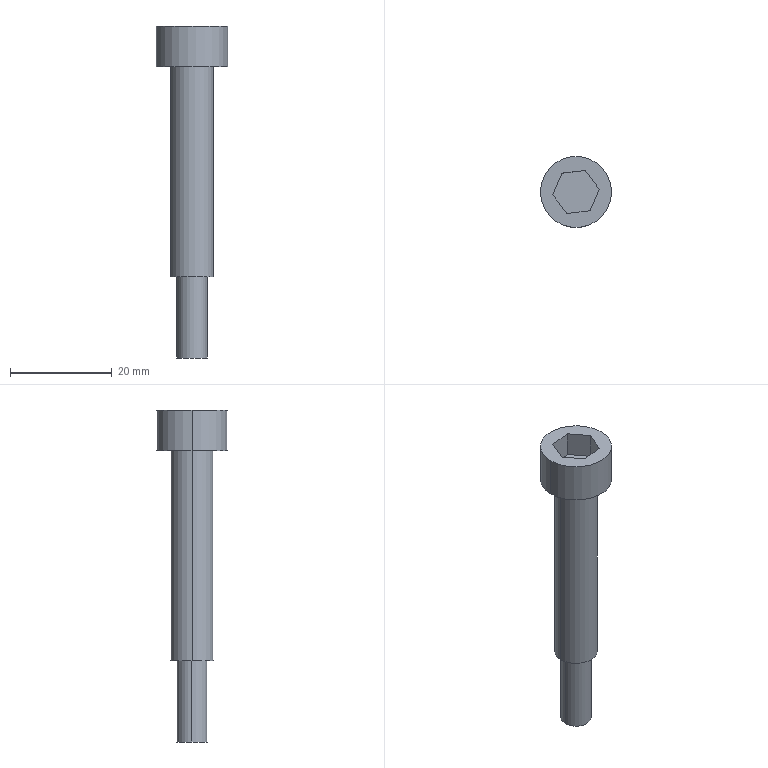Part | SolidWorks | features ICE 2, Cut 1, Extrusion 1 | 1 solid | 17 faces | box 14 x 14 x 65.4 mm | volume 3691 mm3 | plane 11 | cylinder 6 | commonest cylinder face diameters 6 x2 8.382 x2 14 x2
STEP:
#1=CARTESIAN_POINT('',(-29.159,-76.997,-57.4));
#2=VERTEX_POINT('',#1);
#3=CARTESIAN_POINT('',(-23.159,-76.997,-57.4));
#4=VERTEX_POINT('',#3);
#5=CARTESIAN_POINT('',(-26.159,-76.997,-57.4));
#6=DIRECTION('',(0.,0.,-1.));
#7=DIRECTION('',(0.,1.,0.));
#8=AXIS2_PLACEMENT_3D('',#5,#6,#7);
#9=CIRCLE('',#8,3.);
#10=EDGE_CURVE('',#2,#4,#9,.T.);
#11=ORIENTED_EDGE('',*,*,#10,.F.);
#12=CARTESIAN_POINT('',(-29.159,-76.997,-41.4));
#13=VERTEX_POINT('',#12);
#14=CARTESIAN_POINT('',(-29.159,-76.997,-65.885));
#15=DIRECTION('',(0.,0.,1.));
#16=VECTOR('',#15,1000.);
#17=LINE('',#14,#16);
#18=EDGE_CURVE('',#2,#13,#17,.T.);
#19=ORIENTED_EDGE('',*,*,#18,.T.);
#20=CARTESIAN_POINT('',(-23.159,-76.997,-41.4));
#21=VERTEX_POINT('',#20);
#22=CARTESIAN_POINT('',(-26.159,-76.997,-41.4));
#23=DIRECTION('',(0.,0.,-1.));
#24=DIRECTION('',(1.,0.,0.));
#25=AXIS2_PLACEMENT_3D('',#22,#23,#24);
#26=CIRCLE('',#25,3.);
#27=EDGE_CURVE('',#13,#21,#26,.T.);
#28=ORIENTED_EDGE('',*,*,#27,.T.);
#29=CARTESIAN_POINT('',(-23.159,-76.997,-65.885));
#30=DIRECTION('',(0.,0.,1.));
#31=VECTOR('',#30,1000.);
#32=LINE('',#29,#31);
#33=EDGE_CURVE('',#4,#21,#32,.T.);
#34=ORIENTED_EDGE('',*,*,#33,.F.);
#35=EDGE_LOOP('',(#11,#19,#28,#34));
#36=FACE_OUTER_BOUND('',#35,.T.);
#37=CARTESIAN_POINT('',(-26.159,-76.997,-65.885));
#38=DIRECTION('',(0.,0.,1.));
#39=DIRECTION('',(1.,0.,0.));
#40=AXIS2_PLACEMENT_3D('',#37,#38,#39);
#41=CYLINDRICAL_SURFACE('',#40,3.);
#42=ADVANCED_FACE('',(#36),#41,.T.);
#43=CARTESIAN_POINT('',(-21.968,-76.997,-41.4));
#44=VERTEX_POINT('',#43);
#45=CARTESIAN_POINT('',(-30.35,-76.997,-41.4));
#46=VERTEX_POINT('',#45);
#47=CARTESIAN_POINT('',(-26.159,-76.997,-41.4));
#48=DIRECTION('',(0.,0.,1.));
#49=DIRECTION('',(1.,0.,0.));
#50=AXIS2_PLACEMENT_3D('',#47,#48,#49);
#51=CIRCLE('',#50,4.191);
#52=EDGE_CURVE('',#44,#46,#51,.T.);
#53=ORIENTED_EDGE('',*,*,#52,.T.);
#54=CARTESIAN_POINT('',(-30.35,-76.997,0.));
#55=VERTEX_POINT('',#54);
#56=CARTESIAN_POINT('',(-30.35,-76.997,-53.254));
#57=DIRECTION('',(0.,0.,1.));
#58=VECTOR('',#57,1000.);
#59=LINE('',#56,#58);
#60=EDGE_CURVE('',#46,#55,#59,.T.);
#61=ORIENTED_EDGE('',*,*,#60,.T.);
#62=CARTESIAN_POINT('',(-21.968,-76.997,0.));
#63=VERTEX_POINT('',#62);
#64=CARTESIAN_POINT('',(-26.159,-76.997,0.));
#65=DIRECTION('',(0.,0.,-1.));
#66=DIRECTION('',(1.,0.,0.));
#67=AXIS2_PLACEMENT_3D('',#64,#65,#66);
#68=CIRCLE('',#67,4.191);
#69=EDGE_CURVE('',#55,#63,#68,.T.);
#70=ORIENTED_EDGE('',*,*,#69,.T.);
#71=CARTESIAN_POINT('',(-21.968,-76.997,-53.254));
#72=DIRECTION('',(0.,0.,1.));
#73=VECTOR('',#72,1000.);
#74=LINE('',#71,#73);
#75=EDGE_CURVE('',#44,#63,#74,.T.);
#76=ORIENTED_EDGE('',*,*,#75,.F.);
#77=EDGE_LOOP('',(#53,#61,#70,#76));
#78=FACE_OUTER_BOUND('',#77,.T.);
#79=CARTESIAN_POINT('',(-26.159,-76.997,-53.254));
#80=DIRECTION('',(0.,0.,1.));
#81=DIRECTION('',(1.,0.,0.));
#82=AXIS2_PLACEMENT_3D('',#79,#80,#81);
#83=CYLINDRICAL_SURFACE('',#82,4.191);
#84=ADVANCED_FACE('',(#78),#83,.T.);
#85=CARTESIAN_POINT('',(-19.159,-76.997,8.));
#86=VERTEX_POINT('',#85);
#87=CARTESIAN_POINT('',(-33.159,-76.997,8.));
#88=VERTEX_POINT('',#87);
#89=CARTESIAN_POINT('',(-26.159,-76.997,8.));
#90=DIRECTION('',(0.,0.,1.));
#91=DIRECTION('',(1.,0.,0.));
#92=AXIS2_PLACEMENT_3D('',#89,#90,#91);
#93=CIRCLE('',#92,7.);
#94=EDGE_CURVE('',#86,#88,#93,.T.);
#95=ORIENTED_EDGE('',*,*,#94,.F.);
#96=CARTESIAN_POINT('',(-19.159,-76.997,0.));
#97=VERTEX_POINT('',#96);
#98=CARTESIAN_POINT('',(-19.159,-76.997,8.));
#99=DIRECTION('',(0.,0.,-1.));
#100=VECTOR('',#99,1000.);
#101=LINE('',#98,#100);
#102=EDGE_CURVE('',#86,#97,#101,.T.);
#103=ORIENTED_EDGE('',*,*,#102,.T.);
#104=CARTESIAN_POINT('',(-33.159,-76.997,0.));
#105=VERTEX_POINT('',#104);
#106=CARTESIAN_POINT('',(-26.159,-76.997,0.));
#107=DIRECTION('',(0.,0.,1.));
#108=DIRECTION('',(1.,0.,0.));
#109=AXIS2_PLACEMENT_3D('',#106,#107,#108);
#110=CIRCLE('',#109,7.);
#111=EDGE_CURVE('',#97,#105,#110,.T.);
#112=ORIENTED_EDGE('',*,*,#111,.T.);
#113=CARTESIAN_POINT('',(-33.159,-76.997,8.));
#114=DIRECTION('',(0.,0.,-1.));
#115=VECTOR('',#114,1000.);
#116=LINE('',#113,#115);
#117=EDGE_CURVE('',#88,#105,#116,.T.);
#118=ORIENTED_EDGE('',*,*,#117,.F.);
#119=EDGE_LOOP('',(#95,#103,#112,#118));
#120=FACE_OUTER_BOUND('',#119,.T.);
#121=CARTESIAN_POINT('',(-26.159,-76.997,8.));
#122=DIRECTION('',(0.,0.,-1.));
#123=DIRECTION('',(-1.,0.,0.));
#124=AXIS2_PLACEMENT_3D('',#121,#122,#123);
#125=CYLINDRICAL_SURFACE('',#124,7.);
#126=ADVANCED_FACE('',(#120),#125,.T.);
#127=ORIENTED_EDGE('',*,*,#102,.F.);
#128=CARTESIAN_POINT('',(-26.159,-76.997,8.));
#129=DIRECTION('',(0.,0.,1.));
#130=DIRECTION('',(1.,0.,0.));
#131=AXIS2_PLACEMENT_3D('',#128,#129,#130);
#132=CIRCLE('',#131,7.);
#133=EDGE_CURVE('',#88,#86,#132,.T.);
#134=ORIENTED_EDGE('',*,*,#133,.F.);
#135=ORIENTED_EDGE('',*,*,#117,.T.);
#136=CARTESIAN_POINT('',(-26.159,-76.997,0.));
#137=DIRECTION('',(0.,0.,1.));
#138=DIRECTION('',(1.,0.,0.));
#139=AXIS2_PLACEMENT_3D('',#136,#137,#138);
#140=CIRCLE('',#139,7.);
#141=EDGE_CURVE('',#105,#97,#140,.T.);
#142=ORIENTED_EDGE('',*,*,#141,.T.);
#143=EDGE_LOOP('',(#127,#134,#135,#142));
#144=FACE_OUTER_BOUND('',#143,.T.);
#145=CARTESIAN_POINT('',(-26.159,-76.997,8.));
#146=DIRECTION('',(0.,0.,-1.));
#147=DIRECTION('',(-1.,0.,0.));
#148=AXIS2_PLACEMENT_3D('',#145,#146,#147);
#149=CYLINDRICAL_SURFACE('',#148,7.);
#150=ADVANCED_FACE('',(#144),#149,.T.);
#151=CARTESIAN_POINT('',(-21.575,-76.433,8.));
#152=VERTEX_POINT('',#151);
#153=CARTESIAN_POINT('',(-24.356,-72.745,8.));
#154=VERTEX_POINT('',#153);
#155=CARTESIAN_POINT('',(-21.575,-76.433,8.));
#156=DIRECTION('',(-0.6021,0.7984,0.));
#157=VECTOR('',#156,1000.);
#158=LINE('',#155,#157);
#159=EDGE_CURVE('',#152,#154,#158,.T.);
#160=ORIENTED_EDGE('',*,*,#159,.F.);
#161=CARTESIAN_POINT('',(-23.378,-80.685,8.));
#162=VERTEX_POINT('',#161);
#163=CARTESIAN_POINT('',(-23.378,-80.685,8.));
#164=DIRECTION('',(0.3904,0.9206,0.));
#165=VECTOR('',#164,1000.);
#166=LINE('',#163,#165);
#167=EDGE_CURVE('',#162,#152,#166,.T.);
#168=ORIENTED_EDGE('',*,*,#167,.F.);
#169=CARTESIAN_POINT('',(-27.962,-81.25,8.));
#170=VERTEX_POINT('',#169);
#171=CARTESIAN_POINT('',(-27.962,-81.25,8.));
#172=DIRECTION('',(0.9925,0.1222,0.));
#173=VECTOR('',#172,1000.);
#174=LINE('',#171,#173);
#175=EDGE_CURVE('',#170,#162,#174,.T.);
#176=ORIENTED_EDGE('',*,*,#175,.F.);
#177=CARTESIAN_POINT('',(-30.743,-77.562,8.));
#178=VERTEX_POINT('',#177);
#179=CARTESIAN_POINT('',(-30.743,-77.562,8.));
#180=DIRECTION('',(0.6021,-0.7984,0.));
#181=VECTOR('',#180,1000.);
#182=LINE('',#179,#181);
#183=EDGE_CURVE('',#178,#170,#182,.T.);
#184=ORIENTED_EDGE('',*,*,#183,.F.);
#185=CARTESIAN_POINT('',(-28.94,-73.31,8.));
#186=VERTEX_POINT('',#185);
#187=CARTESIAN_POINT('',(-28.94,-73.31,8.));
#188=DIRECTION('',(-0.3904,-0.9206,0.));
#189=VECTOR('',#188,1000.);
#190=LINE('',#187,#189);
#191=EDGE_CURVE('',#186,#178,#190,.T.);
#192=ORIENTED_EDGE('',*,*,#191,.F.);
#193=CARTESIAN_POINT('',(-24.356,-72.745,8.));
#194=DIRECTION('',(-0.9925,-0.1222,0.));
#195=VECTOR('',#194,1000.);
#196=LINE('',#193,#195);
#197=EDGE_CURVE('',#154,#186,#196,.T.);
#198=ORIENTED_EDGE('',*,*,#197,.F.);
#199=EDGE_LOOP('',(#160,#168,#176,#184,#192,#198));
#200=FACE_BOUND('',#199,.T.);
#201=ORIENTED_EDGE('',*,*,#133,.T.);
#202=ORIENTED_EDGE('',*,*,#94,.T.);
#203=EDGE_LOOP('',(#201,#202));
#204=FACE_OUTER_BOUND('',#203,.T.);
#205=CARTESIAN_POINT('',(-26.159,-76.997,8.));
#206=DIRECTION('',(0.,0.,1.));
#207=DIRECTION('',(1.,0.,0.));
#208=AXIS2_PLACEMENT_3D('',#205,#206,#207);
#209=PLANE('',#208);
#210=ADVANCED_FACE('',(#200,#204),#209,.T.);
#211=CARTESIAN_POINT('',(-26.159,-76.997,0.));
#212=DIRECTION('',(0.,0.,-1.));
#213=DIRECTION('',(1.,0.,0.));
#214=AXIS2_PLACEMENT_3D('',#211,#212,#213);
#215=CIRCLE('',#214,4.191);
#216=EDGE_CURVE('',#63,#55,#215,.T.);
#217=ORIENTED_EDGE('',*,*,#216,.F.);
#218=ORIENTED_EDGE('',*,*,#69,.F.);
#219=EDGE_LOOP('',(#217,#218));
#220=FACE_BOUND('',#219,.T.);
#221=ORIENTED_EDGE('',*,*,#141,.F.);
#222=ORIENTED_EDGE('',*,*,#111,.F.);
#223=EDGE_LOOP('',(#221,#222));
#224=FACE_OUTER_BOUND('',#223,.T.);
#225=CARTESIAN_POINT('',(-26.159,-76.997,0.));
#226=DIRECTION('',(0.,0.,1.));
#227=DIRECTION('',(1.,0.,0.));
#228=AXIS2_PLACEMENT_3D('',#225,#226,#227);
#229=PLANE('',#228);
#230=ADVANCED_FACE('',(#220,#224),#229,.F.);
#231=ORIENTED_EDGE('',*,*,#60,.F.);
#232=CARTESIAN_POINT('',(-26.159,-76.997,-41.4));
#233=DIRECTION('',(0.,0.,1.));
#234=DIRECTION('',(1.,0.,0.));
#235=AXIS2_PLACEMENT_3D('',#232,#233,#234);
#236=CIRCLE('',#235,4.191);
#237=EDGE_CURVE('',#46,#44,#236,.T.);
#238=ORIENTED_EDGE('',*,*,#237,.T.);
#239=ORIENTED_EDGE('',*,*,#75,.T.);
#240=ORIENTED_EDGE('',*,*,#216,.T.);
#241=EDGE_LOOP('',(#231,#238,#239,#240));
#242=FACE_OUTER_BOUND('',#241,.T.);
#243=CARTESIAN_POINT('',(-26.159,-76.997,-53.254));
#244=DIRECTION('',(0.,0.,1.));
#245=DIRECTION('',(1.,0.,0.));
#246=AXIS2_PLACEMENT_3D('',#243,#244,#245);
#247=CYLINDRICAL_SURFACE('',#246,4.191);
#248=ADVANCED_FACE('',(#242),#247,.T.);
#249=CARTESIAN_POINT('',(-26.159,-76.997,-41.4));
#250=DIRECTION('',(0.,0.,-1.));
#251=DIRECTION('',(1.,0.,0.));
#252=AXIS2_PLACEMENT_3D('',#249,#250,#251);
#253=CIRCLE('',#252,3.);
#254=EDGE_CURVE('',#21,#13,#253,.T.);
#255=ORIENTED_EDGE('',*,*,#254,.F.);
#256=ORIENTED_EDGE('',*,*,#27,.F.);
#257=EDGE_LOOP('',(#255,#256));
#258=FACE_BOUND('',#257,.T.);
#259=ORIENTED_EDGE('',*,*,#52,.F.);
#260=ORIENTED_EDGE('',*,*,#237,.F.);
#261=EDGE_LOOP('',(#259,#260));
#262=FACE_OUTER_BOUND('',#261,.T.);
#263=CARTESIAN_POINT('',(-26.159,-76.997,-41.4));
#264=DIRECTION('',(0.,0.,1.));
#265=DIRECTION('',(1.,0.,0.));
#266=AXIS2_PLACEMENT_3D('',#263,#264,#265);
#267=PLANE('',#266);
#268=ADVANCED_FACE('',(#258,#262),#267,.F.);
#269=ORIENTED_EDGE('',*,*,#18,.F.);
#270=CARTESIAN_POINT('',(-26.159,-76.997,-57.4));
#271=DIRECTION('',(0.,0.,-1.));
#272=DIRECTION('',(0.,1.,0.));
#273=AXIS2_PLACEMENT_3D('',#270,#271,#272);
#274=CIRCLE('',#273,3.);
#275=EDGE_CURVE('',#4,#2,#274,.T.);
#276=ORIENTED_EDGE('',*,*,#275,.F.);
#277=ORIENTED_EDGE('',*,*,#33,.T.);
#278=ORIENTED_EDGE('',*,*,#254,.T.);
#279=EDGE_LOOP('',(#269,#276,#277,#278));
#280=FACE_OUTER_BOUND('',#279,.T.);
#281=CARTESIAN_POINT('',(-26.159,-76.997,-65.885));
#282=DIRECTION('',(0.,0.,1.));
#283=DIRECTION('',(1.,0.,0.));
#284=AXIS2_PLACEMENT_3D('',#281,#282,#283);
#285=CYLINDRICAL_SURFACE('',#284,3.);
#286=ADVANCED_FACE('',(#280),#285,.T.);
#287=ORIENTED_EDGE('',*,*,#275,.T.);
#288=ORIENTED_EDGE('',*,*,#10,.T.);
#289=EDGE_LOOP('',(#287,#288));
#290=FACE_OUTER_BOUND('',#289,.T.);
#291=CARTESIAN_POINT('',(220.798,92.092,-57.4));
#292=DIRECTION('',(0.,0.,-1.));
#293=DIRECTION('',(0.,1.,0.));
#294=AXIS2_PLACEMENT_3D('',#291,#292,#293);
#295=PLANE('',#294);
#296=ADVANCED_FACE('',(#290),#295,.T.);
#297=ORIENTED_EDGE('',*,*,#159,.T.);
#298=CARTESIAN_POINT('',(-24.356,-72.745,3.));
#299=VERTEX_POINT('',#298);
#300=CARTESIAN_POINT('',(-24.356,-72.745,3.));
#301=DIRECTION('',(0.,0.,1.));
#302=VECTOR('',#301,1000.);
#303=LINE('',#300,#302);
#304=EDGE_CURVE('',#299,#154,#303,.T.);
#305=ORIENTED_EDGE('',*,*,#304,.F.);
#306=CARTESIAN_POINT('',(-21.575,-76.433,3.));
#307=VERTEX_POINT('',#306);
#308=CARTESIAN_POINT('',(-21.575,-76.433,3.));
#309=DIRECTION('',(-0.6021,0.7984,0.));
#310=VECTOR('',#309,1000.);
#311=LINE('',#308,#310);
#312=EDGE_CURVE('',#307,#299,#311,.T.);
#313=ORIENTED_EDGE('',*,*,#312,.F.);
#314=CARTESIAN_POINT('',(-21.575,-76.433,3.));
#315=DIRECTION('',(0.,0.,1.));
#316=VECTOR('',#315,1000.);
#317=LINE('',#314,#316);
#318=EDGE_CURVE('',#307,#152,#317,.T.);
#319=ORIENTED_EDGE('',*,*,#318,.T.);
#320=EDGE_LOOP('',(#297,#305,#313,#319));
#321=FACE_OUTER_BOUND('',#320,.T.);
#322=CARTESIAN_POINT('',(-21.575,-76.433,3.));
#323=DIRECTION('',(0.7984,0.6021,0.));
#324=DIRECTION('',(-0.6021,0.7984,0.));
#325=AXIS2_PLACEMENT_3D('',#322,#323,#324);
#326=PLANE('',#325);
#327=ADVANCED_FACE('',(#321),#326,.F.);
#328=ORIENTED_EDGE('',*,*,#167,.T.);
#329=ORIENTED_EDGE('',*,*,#318,.F.);
#330=CARTESIAN_POINT('',(-23.378,-80.685,3.));
#331=VERTEX_POINT('',#330);
#332=CARTESIAN_POINT('',(-23.378,-80.685,3.));
#333=DIRECTION('',(0.3904,0.9206,0.));
#334=VECTOR('',#333,1000.);
#335=LINE('',#332,#334);
#336=EDGE_CURVE('',#331,#307,#335,.T.);
#337=ORIENTED_EDGE('',*,*,#336,.F.);
#338=CARTESIAN_POINT('',(-23.378,-80.685,3.));
#339=DIRECTION('',(0.,0.,1.));
#340=VECTOR('',#339,1000.);
#341=LINE('',#338,#340);
#342=EDGE_CURVE('',#331,#162,#341,.T.);
#343=ORIENTED_EDGE('',*,*,#342,.T.);
#344=EDGE_LOOP('',(#328,#329,#337,#343));
#345=FACE_OUTER_BOUND('',#344,.T.);
#346=CARTESIAN_POINT('',(-23.378,-80.685,3.));
#347=DIRECTION('',(0.9206,-0.3904,0.));
#348=DIRECTION('',(0.3904,0.9206,0.));
#349=AXIS2_PLACEMENT_3D('',#346,#347,#348);
#350=PLANE('',#349);
#351=ADVANCED_FACE('',(#345),#350,.F.);
#352=ORIENTED_EDGE('',*,*,#175,.T.);
#353=ORIENTED_EDGE('',*,*,#342,.F.);
#354=CARTESIAN_POINT('',(-27.962,-81.25,3.));
#355=VERTEX_POINT('',#354);
#356=CARTESIAN_POINT('',(-27.962,-81.25,3.));
#357=DIRECTION('',(0.9925,0.1222,0.));
#358=VECTOR('',#357,1000.);
#359=LINE('',#356,#358);
#360=EDGE_CURVE('',#355,#331,#359,.T.);
#361=ORIENTED_EDGE('',*,*,#360,.F.);
#362=CARTESIAN_POINT('',(-27.962,-81.25,3.));
#363=DIRECTION('',(0.,0.,1.));
#364=VECTOR('',#363,1000.);
#365=LINE('',#362,#364);
#366=EDGE_CURVE('',#355,#170,#365,.T.);
#367=ORIENTED_EDGE('',*,*,#366,.T.);
#368=EDGE_LOOP('',(#352,#353,#361,#367));
#369=FACE_OUTER_BOUND('',#368,.T.);
#370=CARTESIAN_POINT('',(-27.962,-81.25,3.));
#371=DIRECTION('',(0.1222,-0.9925,0.));
#372=DIRECTION('',(0.9925,0.1222,0.));
#373=AXIS2_PLACEMENT_3D('',#370,#371,#372);
#374=PLANE('',#373);
#375=ADVANCED_FACE('',(#369),#374,.F.);
#376=ORIENTED_EDGE('',*,*,#183,.T.);
#377=ORIENTED_EDGE('',*,*,#366,.F.);
#378=CARTESIAN_POINT('',(-30.743,-77.562,3.));
#379=VERTEX_POINT('',#378);
#380=CARTESIAN_POINT('',(-30.743,-77.562,3.));
#381=DIRECTION('',(0.6021,-0.7984,0.));
#382=VECTOR('',#381,1000.);
#383=LINE('',#380,#382);
#384=EDGE_CURVE('',#379,#355,#383,.T.);
#385=ORIENTED_EDGE('',*,*,#384,.F.);
#386=CARTESIAN_POINT('',(-30.743,-77.562,3.));
#387=DIRECTION('',(0.,0.,1.));
#388=VECTOR('',#387,1000.);
#389=LINE('',#386,#388);
#390=EDGE_CURVE('',#379,#178,#389,.T.);
#391=ORIENTED_EDGE('',*,*,#390,.T.);
#392=EDGE_LOOP('',(#376,#377,#385,#391));
#393=FACE_OUTER_BOUND('',#392,.T.);
#394=CARTESIAN_POINT('',(-30.743,-77.562,3.));
#395=DIRECTION('',(-0.7984,-0.6021,0.));
#396=DIRECTION('',(0.6021,-0.7984,0.));
#397=AXIS2_PLACEMENT_3D('',#394,#395,#396);
#398=PLANE('',#397);
#399=ADVANCED_FACE('',(#393),#398,.F.);
#400=ORIENTED_EDGE('',*,*,#191,.T.);
#401=ORIENTED_EDGE('',*,*,#390,.F.);
#402=CARTESIAN_POINT('',(-28.94,-73.31,3.));
#403=VERTEX_POINT('',#402);
#404=CARTESIAN_POINT('',(-28.94,-73.31,3.));
#405=DIRECTION('',(-0.3904,-0.9206,0.));
#406=VECTOR('',#405,1000.);
#407=LINE('',#404,#406);
#408=EDGE_CURVE('',#403,#379,#407,.T.);
#409=ORIENTED_EDGE('',*,*,#408,.F.);
#410=CARTESIAN_POINT('',(-28.94,-73.31,3.));
#411=DIRECTION('',(0.,0.,1.));
#412=VECTOR('',#411,1000.);
#413=LINE('',#410,#412);
#414=EDGE_CURVE('',#403,#186,#413,.T.);
#415=ORIENTED_EDGE('',*,*,#414,.T.);
#416=EDGE_LOOP('',(#400,#401,#409,#415));
#417=FACE_OUTER_BOUND('',#416,.T.);
#418=CARTESIAN_POINT('',(-28.94,-73.31,3.));
#419=DIRECTION('',(-0.9206,0.3904,0.));
#420=DIRECTION('',(-0.3904,-0.9206,0.));
#421=AXIS2_PLACEMENT_3D('',#418,#419,#420);
#422=PLANE('',#421);
#423=ADVANCED_FACE('',(#417),#422,.F.);
#424=ORIENTED_EDGE('',*,*,#197,.T.);
#425=ORIENTED_EDGE('',*,*,#414,.F.);
#426=CARTESIAN_POINT('',(-24.356,-72.745,3.));
#427=DIRECTION('',(-0.9925,-0.1222,0.));
#428=VECTOR('',#427,1000.);
#429=LINE('',#426,#428);
#430=EDGE_CURVE('',#299,#403,#429,.T.);
#431=ORIENTED_EDGE('',*,*,#430,.F.);
#432=ORIENTED_EDGE('',*,*,#304,.T.);
#433=EDGE_LOOP('',(#424,#425,#431,#432));
#434=FACE_OUTER_BOUND('',#433,.T.);
#435=CARTESIAN_POINT('',(-24.356,-72.745,3.));
#436=DIRECTION('',(-0.1222,0.9925,0.));
#437=DIRECTION('',(-0.9925,-0.1222,0.));
#438=AXIS2_PLACEMENT_3D('',#435,#436,#437);
#439=PLANE('',#438);
#440=ADVANCED_FACE('',(#434),#439,.F.);
#441=ORIENTED_EDGE('',*,*,#312,.T.);
#442=ORIENTED_EDGE('',*,*,#430,.T.);
#443=ORIENTED_EDGE('',*,*,#408,.T.);
#444=ORIENTED_EDGE('',*,*,#384,.T.);
#445=ORIENTED_EDGE('',*,*,#360,.T.);
#446=ORIENTED_EDGE('',*,*,#336,.T.);
#447=EDGE_LOOP('',(#441,#442,#443,#444,#445,#446));
#448=FACE_OUTER_BOUND('',#447,.T.);
#449=CARTESIAN_POINT('',(0.,0.,3.));
#450=DIRECTION('',(0.,0.,1.));
#451=DIRECTION('',(1.,0.,0.));
#452=AXIS2_PLACEMENT_3D('',#449,#450,#451);
#453=PLANE('',#452);
#454=ADVANCED_FACE('',(#448),#453,.T.);
#455=CLOSED_SHELL('',(#42,#84,#126,#150,#210,#230,#248,#268,#286,#296,#327,#351,#375,#399,#423,#440,#454));
#456=MANIFOLD_SOLID_BREP('',#455);
#457=CARTESIAN_POINT('',(0.,0.,0.));
#458=DIRECTION('',(0.,0.,1.));
#459=DIRECTION('',(1.,0.,0.));
#460=AXIS2_PLACEMENT_3D('',#457,#458,#459);
#461=(LENGTH_UNIT()NAMED_UNIT(*)SI_UNIT(.MILLI.,.METRE.));
#462=UNCERTAINTY_MEASURE_WITH_UNIT(LENGTH_MEASURE(0.00001),#461,'','');
#463=(NAMED_UNIT(*)PLANE_ANGLE_UNIT()SI_UNIT($,.RADIAN.));
#464=(NAMED_UNIT(*)SI_UNIT($,.STERADIAN.)SOLID_ANGLE_UNIT());
#465=(GEOMETRIC_REPRESENTATION_CONTEXT(3)GLOBAL_UNCERTAINTY_ASSIGNED_CONTEXT((#462))GLOBAL_UNIT_ASSIGNED_CONTEXT((#461,#463,#464))REPRESENTATION_CONTEXT('',''));
#466=ADVANCED_BREP_SHAPE_REPRESENTATION('',(#456,#460),#465);